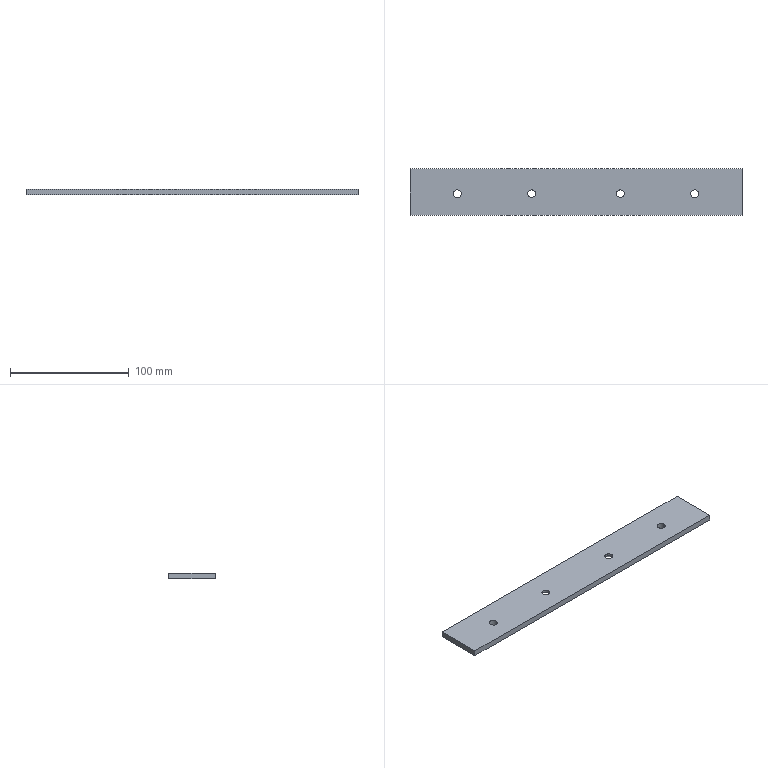Part | STEP file | 44-02-07 Ear Forming Push Plate B | 1 solid | 18 faces | box 280 x 39 x 5 mm | volume 53633 mm3 | cylinder 8 | plane 6 | cone 4 | commonest cylinder face diameters 6.6 x4 6.8 x4
STEP:
#1=CARTESIAN_POINT('',(0.,0.,0.));
#2=DIRECTION('',(0.,0.,1.));
#3=DIRECTION('',(1.,0.,0.));
#4=AXIS2_PLACEMENT_3D('',#1,#2,#3);
#5=CARTESIAN_POINT('',(34.2,0.,0.6));
#6=VERTEX_POINT('',#5);
#7=CARTESIAN_POINT('',(31.1,0.,-2.5));
#8=VERTEX_POINT('',#7);
#9=CARTESIAN_POINT('',(31.1,0.,-2.5));
#10=DIRECTION('',(-0.7071,0.,-0.7071));
#11=VECTOR('',#10,1.);
#12=LINE('',#9,#11);
#13=CARTESIAN_POINT('',(37.5,0.,-2.5));
#14=DIRECTION('',(0.,0.,-1.));
#15=DIRECTION('',(-1.,0.,0.));
#16=AXIS2_PLACEMENT_3D('',#13,#14,#15);
#17=CONICAL_SURFACE('',#16,6.4,0.7854);
#18=CARTESIAN_POINT('',(6.283,0.));
#19=DIRECTION('',(0.,1.));
#20=VECTOR('',#19,1.);
#21=LINE('',#18,#20);
#22=(GEOMETRIC_REPRESENTATION_CONTEXT(2)PARAMETRIC_REPRESENTATION_CONTEXT()REPRESENTATION_CONTEXT('',''));
#23=DEFINITIONAL_REPRESENTATION('',(#21),#22);
#24=PCURVE('',#17,#23);
#25=CARTESIAN_POINT('',(37.5,0.,-2.5));
#26=DIRECTION('',(0.,0.,-1.));
#27=DIRECTION('',(-1.,0.,0.));
#28=AXIS2_PLACEMENT_3D('',#25,#26,#27);
#29=CONICAL_SURFACE('',#28,6.4,0.7854);
#30=CARTESIAN_POINT('',(0.,0.));
#31=DIRECTION('',(0.,1.));
#32=VECTOR('',#31,1.);
#33=LINE('',#30,#32);
#34=(GEOMETRIC_REPRESENTATION_CONTEXT(2)PARAMETRIC_REPRESENTATION_CONTEXT()REPRESENTATION_CONTEXT('',''));
#35=DEFINITIONAL_REPRESENTATION('',(#33),#34);
#36=PCURVE('',#29,#35);
#37=SURFACE_CURVE('',#12,(#24,#36),.PCURVE_S1.);
#38=EDGE_CURVE('',#6,#8,#37,.T.);
#39=ORIENTED_EDGE('',*,*,#38,.T.);
#40=CARTESIAN_POINT('',(43.9,0.,-2.5));
#41=VERTEX_POINT('',#40);
#42=CARTESIAN_POINT('',(37.5,0.,-2.5));
#43=DIRECTION('',(0.,0.,-1.));
#44=DIRECTION('',(-1.,0.,0.));
#45=AXIS2_PLACEMENT_3D('',#42,#43,#44);
#46=CIRCLE('',#45,6.4);
#47=CARTESIAN_POINT('',(0.,0.));
#48=DIRECTION('',(1.,0.));
#49=VECTOR('',#48,1.);
#50=LINE('',#47,#49);
#51=(GEOMETRIC_REPRESENTATION_CONTEXT(2)PARAMETRIC_REPRESENTATION_CONTEXT()REPRESENTATION_CONTEXT('',''));
#52=DEFINITIONAL_REPRESENTATION('',(#50),#51);
#53=PCURVE('',#17,#52);
#54=CARTESIAN_POINT('',(140.,-18.,-2.5));
#55=DIRECTION('',(0.,0.,1.));
#56=DIRECTION('',(1.,0.,0.));
#57=AXIS2_PLACEMENT_3D('',#54,#55,#56);
#58=PLANE('',#57);
#59=CARTESIAN_POINT('',(-108.9,18.));
#60=CARTESIAN_POINT('',(-108.9,29.085));
#61=CARTESIAN_POINT('',(-99.3,23.543));
#62=CARTESIAN_POINT('',(-89.7,18.));
#63=CARTESIAN_POINT('',(-99.3,12.457));
#64=CARTESIAN_POINT('',(-108.9,6.915));
#65=CARTESIAN_POINT('',(-108.9,18.));
#66=(BOUNDED_CURVE()B_SPLINE_CURVE(2,(#59,#60,#61,#62,#63,#64,#65),.UNSPECIFIED.,.T.,.F.)B_SPLINE_CURVE_WITH_KNOTS((1,2,2,2,2,1),(-2.094,0.,2.094,4.189,6.283,8.378),.UNSPECIFIED.)CURVE()GEOMETRIC_REPRESENTATION_ITEM()RATIONAL_B_SPLINE_CURVE((1.,0.5,1.,0.5,1.,0.5,1.))REPRESENTATION_ITEM(''));
#67=(GEOMETRIC_REPRESENTATION_CONTEXT(2)PARAMETRIC_REPRESENTATION_CONTEXT()REPRESENTATION_CONTEXT('',''));
#68=DEFINITIONAL_REPRESENTATION('',(#66),#67);
#69=PCURVE('',#58,#68);
#70=SURFACE_CURVE('',#46,(#53,#69),.PCURVE_S1.);
#71=EDGE_CURVE('',#41,#8,#70,.T.);
#72=ORIENTED_EDGE('',*,*,#71,.F.);
#73=CARTESIAN_POINT('',(40.8,0.,0.6));
#74=VERTEX_POINT('',#73);
#75=CARTESIAN_POINT('',(43.9,0.,-2.5));
#76=DIRECTION('',(0.7071,0.,-0.7071));
#77=VECTOR('',#76,1.);
#78=LINE('',#75,#77);
#79=CARTESIAN_POINT('',(3.142,0.));
#80=DIRECTION('',(0.,1.));
#81=VECTOR('',#80,1.);
#82=LINE('',#79,#81);
#83=(GEOMETRIC_REPRESENTATION_CONTEXT(2)PARAMETRIC_REPRESENTATION_CONTEXT()REPRESENTATION_CONTEXT('',''));
#84=DEFINITIONAL_REPRESENTATION('',(#82),#83);
#85=PCURVE('',#17,#84);
#86=CARTESIAN_POINT('',(3.142,0.));
#87=DIRECTION('',(0.,1.));
#88=VECTOR('',#87,1.);
#89=LINE('',#86,#88);
#90=(GEOMETRIC_REPRESENTATION_CONTEXT(2)PARAMETRIC_REPRESENTATION_CONTEXT()REPRESENTATION_CONTEXT('',''));
#91=DEFINITIONAL_REPRESENTATION('',(#89),#90);
#92=PCURVE('',#29,#91);
#93=SURFACE_CURVE('',#78,(#85,#92),.PCURVE_S1.);
#94=EDGE_CURVE('',#74,#41,#93,.T.);
#95=ORIENTED_EDGE('',*,*,#94,.F.);
#96=CARTESIAN_POINT('',(37.5,0.,0.6));
#97=DIRECTION('',(0.,0.,-1.));
#98=DIRECTION('',(-1.,0.,0.));
#99=AXIS2_PLACEMENT_3D('',#96,#97,#98);
#100=CIRCLE('',#99,3.3);
#101=CARTESIAN_POINT('',(0.,-3.1));
#102=DIRECTION('',(1.,0.));
#103=VECTOR('',#102,1.);
#104=LINE('',#101,#103);
#105=(GEOMETRIC_REPRESENTATION_CONTEXT(2)PARAMETRIC_REPRESENTATION_CONTEXT()REPRESENTATION_CONTEXT('',''));
#106=DEFINITIONAL_REPRESENTATION('',(#104),#105);
#107=PCURVE('',#17,#106);
#108=CARTESIAN_POINT('',(37.5,0.,-2.5));
#109=DIRECTION('',(0.,0.,-1.));
#110=DIRECTION('',(-1.,0.,0.));
#111=AXIS2_PLACEMENT_3D('',#108,#109,#110);
#112=CYLINDRICAL_SURFACE('',#111,3.3);
#113=CARTESIAN_POINT('',(0.,-3.1));
#114=DIRECTION('',(1.,0.));
#115=VECTOR('',#114,1.);
#116=LINE('',#113,#115);
#117=(GEOMETRIC_REPRESENTATION_CONTEXT(2)PARAMETRIC_REPRESENTATION_CONTEXT()REPRESENTATION_CONTEXT('',''));
#118=DEFINITIONAL_REPRESENTATION('',(#116),#117);
#119=PCURVE('',#112,#118);
#120=SURFACE_CURVE('',#100,(#107,#119),.PCURVE_S1.);
#121=EDGE_CURVE('',#74,#6,#120,.T.);
#122=ORIENTED_EDGE('',*,*,#121,.T.);
#123=EDGE_LOOP('',(#39,#72,#95,#122));
#124=FACE_BOUND('',#123,.F.);
#125=ADVANCED_FACE('',(#124),#17,.F.);
#126=CARTESIAN_POINT('',(34.2,0.,2.5));
#127=VERTEX_POINT('',#126);
#128=CARTESIAN_POINT('',(34.2,0.,-2.5));
#129=DIRECTION('',(0.,0.,-1.));
#130=VECTOR('',#129,1.);
#131=LINE('',#128,#130);
#132=CARTESIAN_POINT('',(6.283,0.));
#133=DIRECTION('',(0.,1.));
#134=VECTOR('',#133,1.);
#135=LINE('',#132,#134);
#136=(GEOMETRIC_REPRESENTATION_CONTEXT(2)PARAMETRIC_REPRESENTATION_CONTEXT()REPRESENTATION_CONTEXT('',''));
#137=DEFINITIONAL_REPRESENTATION('',(#135),#136);
#138=PCURVE('',#112,#137);
#139=CARTESIAN_POINT('',(37.5,0.,-2.5));
#140=DIRECTION('',(0.,0.,-1.));
#141=DIRECTION('',(-1.,0.,0.));
#142=AXIS2_PLACEMENT_3D('',#139,#140,#141);
#143=CYLINDRICAL_SURFACE('',#142,3.3);
#144=CARTESIAN_POINT('',(0.,0.));
#145=DIRECTION('',(0.,1.));
#146=VECTOR('',#145,1.);
#147=LINE('',#144,#146);
#148=(GEOMETRIC_REPRESENTATION_CONTEXT(2)PARAMETRIC_REPRESENTATION_CONTEXT()REPRESENTATION_CONTEXT('',''));
#149=DEFINITIONAL_REPRESENTATION('',(#147),#148);
#150=PCURVE('',#143,#149);
#151=SURFACE_CURVE('',#131,(#138,#150),.PCURVE_S1.);
#152=EDGE_CURVE('',#127,#6,#151,.T.);
#153=ORIENTED_EDGE('',*,*,#152,.T.);
#154=ORIENTED_EDGE('',*,*,#121,.F.);
#155=CARTESIAN_POINT('',(40.8,0.,2.5));
#156=VERTEX_POINT('',#155);
#157=CARTESIAN_POINT('',(40.8,0.,-2.5));
#158=DIRECTION('',(0.,0.,-1.));
#159=VECTOR('',#158,1.);
#160=LINE('',#157,#159);
#161=CARTESIAN_POINT('',(3.142,0.));
#162=DIRECTION('',(0.,1.));
#163=VECTOR('',#162,1.);
#164=LINE('',#161,#163);
#165=(GEOMETRIC_REPRESENTATION_CONTEXT(2)PARAMETRIC_REPRESENTATION_CONTEXT()REPRESENTATION_CONTEXT('',''));
#166=DEFINITIONAL_REPRESENTATION('',(#164),#165);
#167=PCURVE('',#112,#166);
#168=CARTESIAN_POINT('',(3.142,0.));
#169=DIRECTION('',(0.,1.));
#170=VECTOR('',#169,1.);
#171=LINE('',#168,#170);
#172=(GEOMETRIC_REPRESENTATION_CONTEXT(2)PARAMETRIC_REPRESENTATION_CONTEXT()REPRESENTATION_CONTEXT('',''));
#173=DEFINITIONAL_REPRESENTATION('',(#171),#172);
#174=PCURVE('',#143,#173);
#175=SURFACE_CURVE('',#160,(#167,#174),.PCURVE_S1.);
#176=EDGE_CURVE('',#156,#74,#175,.T.);
#177=ORIENTED_EDGE('',*,*,#176,.F.);
#178=CARTESIAN_POINT('',(37.5,0.,2.5));
#179=DIRECTION('',(0.,0.,-1.));
#180=DIRECTION('',(-1.,0.,0.));
#181=AXIS2_PLACEMENT_3D('',#178,#179,#180);
#182=CIRCLE('',#181,3.3);
#183=CARTESIAN_POINT('',(0.,-5.));
#184=DIRECTION('',(1.,0.));
#185=VECTOR('',#184,1.);
#186=LINE('',#183,#185);
#187=(GEOMETRIC_REPRESENTATION_CONTEXT(2)PARAMETRIC_REPRESENTATION_CONTEXT()REPRESENTATION_CONTEXT('',''));
#188=DEFINITIONAL_REPRESENTATION('',(#186),#187);
#189=PCURVE('',#112,#188);
#190=CARTESIAN_POINT('',(140.,-18.,2.5));
#191=DIRECTION('',(0.,0.,1.));
#192=DIRECTION('',(1.,0.,0.));
#193=AXIS2_PLACEMENT_3D('',#190,#191,#192);
#194=PLANE('',#193);
#195=CARTESIAN_POINT('',(-105.8,18.));
#196=CARTESIAN_POINT('',(-105.8,23.716));
#197=CARTESIAN_POINT('',(-100.85,20.858));
#198=CARTESIAN_POINT('',(-95.9,18.));
#199=CARTESIAN_POINT('',(-100.85,15.142));
#200=CARTESIAN_POINT('',(-105.8,12.284));
#201=CARTESIAN_POINT('',(-105.8,18.));
#202=(BOUNDED_CURVE()B_SPLINE_CURVE(2,(#195,#196,#197,#198,#199,#200,#201),.UNSPECIFIED.,.T.,.F.)B_SPLINE_CURVE_WITH_KNOTS((1,2,2,2,2,1),(-2.094,0.,2.094,4.189,6.283,8.378),.UNSPECIFIED.)CURVE()GEOMETRIC_REPRESENTATION_ITEM()RATIONAL_B_SPLINE_CURVE((1.,0.5,1.,0.5,1.,0.5,1.))REPRESENTATION_ITEM(''));
#203=(GEOMETRIC_REPRESENTATION_CONTEXT(2)PARAMETRIC_REPRESENTATION_CONTEXT()REPRESENTATION_CONTEXT('',''));
#204=DEFINITIONAL_REPRESENTATION('',(#202),#203);
#205=PCURVE('',#194,#204);
#206=SURFACE_CURVE('',#182,(#189,#205),.PCURVE_S1.);
#207=EDGE_CURVE('',#156,#127,#206,.T.);
#208=ORIENTED_EDGE('',*,*,#207,.T.);
#209=EDGE_LOOP('',(#153,#154,#177,#208));
#210=FACE_BOUND('',#209,.F.);
#211=ADVANCED_FACE('',(#210),#112,.F.);
#212=CARTESIAN_POINT('',(-40.8,0.,0.6));
#213=VERTEX_POINT('',#212);
#214=CARTESIAN_POINT('',(-43.9,0.,-2.5));
#215=VERTEX_POINT('',#214);
#216=CARTESIAN_POINT('',(-43.9,0.,-2.5));
#217=DIRECTION('',(-0.7071,0.,-0.7071));
#218=VECTOR('',#217,1.);
#219=LINE('',#216,#218);
#220=CARTESIAN_POINT('',(-37.5,0.,-2.5));
#221=DIRECTION('',(0.,0.,-1.));
#222=DIRECTION('',(-1.,0.,0.));
#223=AXIS2_PLACEMENT_3D('',#220,#221,#222);
#224=CONICAL_SURFACE('',#223,6.4,0.7854);
#225=CARTESIAN_POINT('',(6.283,0.));
#226=DIRECTION('',(0.,1.));
#227=VECTOR('',#226,1.);
#228=LINE('',#225,#227);
#229=(GEOMETRIC_REPRESENTATION_CONTEXT(2)PARAMETRIC_REPRESENTATION_CONTEXT()REPRESENTATION_CONTEXT('',''));
#230=DEFINITIONAL_REPRESENTATION('',(#228),#229);
#231=PCURVE('',#224,#230);
#232=CARTESIAN_POINT('',(-37.5,0.,-2.5));
#233=DIRECTION('',(0.,0.,-1.));
#234=DIRECTION('',(-1.,0.,0.));
#235=AXIS2_PLACEMENT_3D('',#232,#233,#234);
#236=CONICAL_SURFACE('',#235,6.4,0.7854);
#237=CARTESIAN_POINT('',(0.,0.));
#238=DIRECTION('',(0.,1.));
#239=VECTOR('',#238,1.);
#240=LINE('',#237,#239);
#241=(GEOMETRIC_REPRESENTATION_CONTEXT(2)PARAMETRIC_REPRESENTATION_CONTEXT()REPRESENTATION_CONTEXT('',''));
#242=DEFINITIONAL_REPRESENTATION('',(#240),#241);
#243=PCURVE('',#236,#242);
#244=SURFACE_CURVE('',#219,(#231,#243),.PCURVE_S1.);
#245=EDGE_CURVE('',#213,#215,#244,.T.);
#246=ORIENTED_EDGE('',*,*,#245,.T.);
#247=CARTESIAN_POINT('',(-31.1,0.,-2.5));
#248=VERTEX_POINT('',#247);
#249=CARTESIAN_POINT('',(-37.5,0.,-2.5));
#250=DIRECTION('',(0.,0.,-1.));
#251=DIRECTION('',(-1.,0.,0.));
#252=AXIS2_PLACEMENT_3D('',#249,#250,#251);
#253=CIRCLE('',#252,6.4);
#254=CARTESIAN_POINT('',(0.,0.));
#255=DIRECTION('',(1.,0.));
#256=VECTOR('',#255,1.);
#257=LINE('',#254,#256);
#258=(GEOMETRIC_REPRESENTATION_CONTEXT(2)PARAMETRIC_REPRESENTATION_CONTEXT()REPRESENTATION_CONTEXT('',''));
#259=DEFINITIONAL_REPRESENTATION('',(#257),#258);
#260=PCURVE('',#224,#259);
#261=CARTESIAN_POINT('',(-183.9,18.));
#262=CARTESIAN_POINT('',(-183.9,29.085));
#263=CARTESIAN_POINT('',(-174.3,23.543));
#264=CARTESIAN_POINT('',(-164.7,18.));
#265=CARTESIAN_POINT('',(-174.3,12.457));
#266=CARTESIAN_POINT('',(-183.9,6.915));
#267=CARTESIAN_POINT('',(-183.9,18.));
#268=(BOUNDED_CURVE()B_SPLINE_CURVE(2,(#261,#262,#263,#264,#265,#266,#267),.UNSPECIFIED.,.T.,.F.)B_SPLINE_CURVE_WITH_KNOTS((1,2,2,2,2,1),(-2.094,0.,2.094,4.189,6.283,8.378),.UNSPECIFIED.)CURVE()GEOMETRIC_REPRESENTATION_ITEM()RATIONAL_B_SPLINE_CURVE((1.,0.5,1.,0.5,1.,0.5,1.))REPRESENTATION_ITEM(''));
#269=(GEOMETRIC_REPRESENTATION_CONTEXT(2)PARAMETRIC_REPRESENTATION_CONTEXT()REPRESENTATION_CONTEXT('',''));
#270=DEFINITIONAL_REPRESENTATION('',(#268),#269);
#271=PCURVE('',#58,#270);
#272=SURFACE_CURVE('',#253,(#260,#271),.PCURVE_S1.);
#273=EDGE_CURVE('',#248,#215,#272,.T.);
#274=ORIENTED_EDGE('',*,*,#273,.F.);
#275=CARTESIAN_POINT('',(-34.2,0.,0.6));
#276=VERTEX_POINT('',#275);
#277=CARTESIAN_POINT('',(-31.1,0.,-2.5));
#278=DIRECTION('',(0.7071,0.,-0.7071));
#279=VECTOR('',#278,1.);
#280=LINE('',#277,#279);
#281=CARTESIAN_POINT('',(3.142,0.));
#282=DIRECTION('',(0.,1.));
#283=VECTOR('',#282,1.);
#284=LINE('',#281,#283);
#285=(GEOMETRIC_REPRESENTATION_CONTEXT(2)PARAMETRIC_REPRESENTATION_CONTEXT()REPRESENTATION_CONTEXT('',''));
#286=DEFINITIONAL_REPRESENTATION('',(#284),#285);
#287=PCURVE('',#224,#286);
#288=CARTESIAN_POINT('',(3.142,0.));
#289=DIRECTION('',(0.,1.));
#290=VECTOR('',#289,1.);
#291=LINE('',#288,#290);
#292=(GEOMETRIC_REPRESENTATION_CONTEXT(2)PARAMETRIC_REPRESENTATION_CONTEXT()REPRESENTATION_CONTEXT('',''));
#293=DEFINITIONAL_REPRESENTATION('',(#291),#292);
#294=PCURVE('',#236,#293);
#295=SURFACE_CURVE('',#280,(#287,#294),.PCURVE_S1.);
#296=EDGE_CURVE('',#276,#248,#295,.T.);
#297=ORIENTED_EDGE('',*,*,#296,.F.);
#298=CARTESIAN_POINT('',(-37.5,0.,0.6));
#299=DIRECTION('',(0.,0.,-1.));
#300=DIRECTION('',(-1.,0.,0.));
#301=AXIS2_PLACEMENT_3D('',#298,#299,#300);
#302=CIRCLE('',#301,3.3);
#303=CARTESIAN_POINT('',(0.,-3.1));
#304=DIRECTION('',(1.,0.));
#305=VECTOR('',#304,1.);
#306=LINE('',#303,#305);
#307=(GEOMETRIC_REPRESENTATION_CONTEXT(2)PARAMETRIC_REPRESENTATION_CONTEXT()REPRESENTATION_CONTEXT('',''));
#308=DEFINITIONAL_REPRESENTATION('',(#306),#307);
#309=PCURVE('',#224,#308);
#310=CARTESIAN_POINT('',(-37.5,0.,-2.5));
#311=DIRECTION('',(0.,0.,-1.));
#312=DIRECTION('',(-1.,0.,0.));
#313=AXIS2_PLACEMENT_3D('',#310,#311,#312);
#314=CYLINDRICAL_SURFACE('',#313,3.3);
#315=CARTESIAN_POINT('',(0.,-3.1));
#316=DIRECTION('',(1.,0.));
#317=VECTOR('',#316,1.);
#318=LINE('',#315,#317);
#319=(GEOMETRIC_REPRESENTATION_CONTEXT(2)PARAMETRIC_REPRESENTATION_CONTEXT()REPRESENTATION_CONTEXT('',''));
#320=DEFINITIONAL_REPRESENTATION('',(#318),#319);
#321=PCURVE('',#314,#320);
#322=SURFACE_CURVE('',#302,(#309,#321),.PCURVE_S1.);
#323=EDGE_CURVE('',#276,#213,#322,.T.);
#324=ORIENTED_EDGE('',*,*,#323,.T.);
#325=EDGE_LOOP('',(#246,#274,#297,#324));
#326=FACE_BOUND('',#325,.F.);
#327=ADVANCED_FACE('',(#326),#224,.F.);
#328=CARTESIAN_POINT('',(-40.8,0.,2.5));
#329=VERTEX_POINT('',#328);
#330=CARTESIAN_POINT('',(-40.8,0.,-2.5));
#331=DIRECTION('',(0.,0.,-1.));
#332=VECTOR('',#331,1.);
#333=LINE('',#330,#332);
#334=CARTESIAN_POINT('',(6.283,0.));
#335=DIRECTION('',(0.,1.));
#336=VECTOR('',#335,1.);
#337=LINE('',#334,#336);
#338=(GEOMETRIC_REPRESENTATION_CONTEXT(2)PARAMETRIC_REPRESENTATION_CONTEXT()REPRESENTATION_CONTEXT('',''));
#339=DEFINITIONAL_REPRESENTATION('',(#337),#338);
#340=PCURVE('',#314,#339);
#341=CARTESIAN_POINT('',(-37.5,0.,-2.5));
#342=DIRECTION('',(0.,0.,-1.));
#343=DIRECTION('',(-1.,0.,0.));
#344=AXIS2_PLACEMENT_3D('',#341,#342,#343);
#345=CYLINDRICAL_SURFACE('',#344,3.3);
#346=CARTESIAN_POINT('',(0.,0.));
#347=DIRECTION('',(0.,1.));
#348=VECTOR('',#347,1.);
#349=LINE('',#346,#348);
#350=(GEOMETRIC_REPRESENTATION_CONTEXT(2)PARAMETRIC_REPRESENTATION_CONTEXT()REPRESENTATION_CONTEXT('',''));
#351=DEFINITIONAL_REPRESENTATION('',(#349),#350);
#352=PCURVE('',#345,#351);
#353=SURFACE_CURVE('',#333,(#340,#352),.PCURVE_S1.);
#354=EDGE_CURVE('',#329,#213,#353,.T.);
#355=ORIENTED_EDGE('',*,*,#354,.T.);
#356=ORIENTED_EDGE('',*,*,#323,.F.);
#357=CARTESIAN_POINT('',(-34.2,0.,2.5));
#358=VERTEX_POINT('',#357);
#359=CARTESIAN_POINT('',(-34.2,0.,-2.5));
#360=DIRECTION('',(0.,0.,-1.));
#361=VECTOR('',#360,1.);
#362=LINE('',#359,#361);
#363=CARTESIAN_POINT('',(3.142,0.));
#364=DIRECTION('',(0.,1.));
#365=VECTOR('',#364,1.);
#366=LINE('',#363,#365);
#367=(GEOMETRIC_REPRESENTATION_CONTEXT(2)PARAMETRIC_REPRESENTATION_CONTEXT()REPRESENTATION_CONTEXT('',''));
#368=DEFINITIONAL_REPRESENTATION('',(#366),#367);
#369=PCURVE('',#314,#368);
#370=CARTESIAN_POINT('',(3.142,0.));
#371=DIRECTION('',(0.,1.));
#372=VECTOR('',#371,1.);
#373=LINE('',#370,#372);
#374=(GEOMETRIC_REPRESENTATION_CONTEXT(2)PARAMETRIC_REPRESENTATION_CONTEXT()REPRESENTATION_CONTEXT('',''));
#375=DEFINITIONAL_REPRESENTATION('',(#373),#374);
#376=PCURVE('',#345,#375);
#377=SURFACE_CURVE('',#362,(#369,#376),.PCURVE_S1.);
#378=EDGE_CURVE('',#358,#276,#377,.T.);
#379=ORIENTED_EDGE('',*,*,#378,.F.);
#380=CARTESIAN_POINT('',(-37.5,0.,2.5));
#381=DIRECTION('',(0.,0.,-1.));
#382=DIRECTION('',(-1.,0.,0.));
#383=AXIS2_PLACEMENT_3D('',#380,#381,#382);
#384=CIRCLE('',#383,3.3);
#385=CARTESIAN_POINT('',(0.,-5.));
#386=DIRECTION('',(1.,0.));
#387=VECTOR('',#386,1.);
#388=LINE('',#385,#387);
#389=(GEOMETRIC_REPRESENTATION_CONTEXT(2)PARAMETRIC_REPRESENTATION_CONTEXT()REPRESENTATION_CONTEXT('',''));
#390=DEFINITIONAL_REPRESENTATION('',(#388),#389);
#391=PCURVE('',#314,#390);
#392=CARTESIAN_POINT('',(-180.8,18.));
#393=CARTESIAN_POINT('',(-180.8,23.716));
#394=CARTESIAN_POINT('',(-175.85,20.858));
#395=CARTESIAN_POINT('',(-170.9,18.));
#396=CARTESIAN_POINT('',(-175.85,15.142));
#397=CARTESIAN_POINT('',(-180.8,12.284));
#398=CARTESIAN_POINT('',(-180.8,18.));
#399=(BOUNDED_CURVE()B_SPLINE_CURVE(2,(#392,#393,#394,#395,#396,#397,#398),.UNSPECIFIED.,.T.,.F.)B_SPLINE_CURVE_WITH_KNOTS((1,2,2,2,2,1),(-2.094,0.,2.094,4.189,6.283,8.378),.UNSPECIFIED.)CURVE()GEOMETRIC_REPRESENTATION_ITEM()RATIONAL_B_SPLINE_CURVE((1.,0.5,1.,0.5,1.,0.5,1.))REPRESENTATION_ITEM(''));
#400=(GEOMETRIC_REPRESENTATION_CONTEXT(2)PARAMETRIC_REPRESENTATION_CONTEXT()REPRESENTATION_CONTEXT('',''));
#401=DEFINITIONAL_REPRESENTATION('',(#399),#400);
#402=PCURVE('',#194,#401);
#403=SURFACE_CURVE('',#384,(#391,#402),.PCURVE_S1.);
#404=EDGE_CURVE('',#358,#329,#403,.T.);
#405=ORIENTED_EDGE('',*,*,#404,.T.);
#406=EDGE_LOOP('',(#355,#356,#379,#405));
#407=FACE_BOUND('',#406,.F.);
#408=ADVANCED_FACE('',(#407),#314,.F.);
#409=CARTESIAN_POINT('',(-103.4,0.,2.5));
#410=VERTEX_POINT('',#409);
#411=CARTESIAN_POINT('',(-103.4,0.,-2.5));
#412=VERTEX_POINT('',#411);
#413=CARTESIAN_POINT('',(-103.4,0.,-2.5));
#414=DIRECTION('',(0.,0.,-1.));
#415=VECTOR('',#414,1.);
#416=LINE('',#413,#415);
#417=CARTESIAN_POINT('',(-100.,0.,-2.5));
#418=DIRECTION('',(0.,0.,-1.));
#419=DIRECTION('',(-1.,0.,0.));
#420=AXIS2_PLACEMENT_3D('',#417,#418,#419);
#421=CYLINDRICAL_SURFACE('',#420,3.4);
#422=CARTESIAN_POINT('',(6.283,0.));
#423=DIRECTION('',(0.,1.));
#424=VECTOR('',#423,1.);
#425=LINE('',#422,#424);
#426=(GEOMETRIC_REPRESENTATION_CONTEXT(2)PARAMETRIC_REPRESENTATION_CONTEXT()REPRESENTATION_CONTEXT('',''));
#427=DEFINITIONAL_REPRESENTATION('',(#425),#426);
#428=PCURVE('',#421,#427);
#429=CARTESIAN_POINT('',(-100.,0.,-2.5));
#430=DIRECTION('',(0.,0.,-1.));
#431=DIRECTION('',(-1.,0.,0.));
#432=AXIS2_PLACEMENT_3D('',#429,#430,#431);
#433=CYLINDRICAL_SURFACE('',#432,3.4);
#434=CARTESIAN_POINT('',(0.,0.));
#435=DIRECTION('',(0.,1.));
#436=VECTOR('',#435,1.);
#437=LINE('',#434,#436);
#438=(GEOMETRIC_REPRESENTATION_CONTEXT(2)PARAMETRIC_REPRESENTATION_CONTEXT()REPRESENTATION_CONTEXT('',''));
#439=DEFINITIONAL_REPRESENTATION('',(#437),#438);
#440=PCURVE('',#433,#439);
#441=SURFACE_CURVE('',#416,(#428,#440),.PCURVE_S1.);
#442=EDGE_CURVE('',#410,#412,#441,.T.);
#443=ORIENTED_EDGE('',*,*,#442,.T.);
#444=CARTESIAN_POINT('',(-96.6,0.,-2.5));
#445=VERTEX_POINT('',#444);
#446=CARTESIAN_POINT('',(-100.,0.,-2.5));
#447=DIRECTION('',(0.,0.,-1.));
#448=DIRECTION('',(-1.,0.,0.));
#449=AXIS2_PLACEMENT_3D('',#446,#447,#448);
#450=CIRCLE('',#449,3.4);
#451=CARTESIAN_POINT('',(0.,0.));
#452=DIRECTION('',(1.,0.));
#453=VECTOR('',#452,1.);
#454=LINE('',#451,#453);
#455=(GEOMETRIC_REPRESENTATION_CONTEXT(2)PARAMETRIC_REPRESENTATION_CONTEXT()REPRESENTATION_CONTEXT('',''));
#456=DEFINITIONAL_REPRESENTATION('',(#454),#455);
#457=PCURVE('',#421,#456);
#458=CARTESIAN_POINT('',(-243.4,18.));
#459=CARTESIAN_POINT('',(-243.4,23.889));
#460=CARTESIAN_POINT('',(-238.3,20.944));
#461=CARTESIAN_POINT('',(-233.2,18.));
#462=CARTESIAN_POINT('',(-238.3,15.056));
#463=CARTESIAN_POINT('',(-243.4,12.111));
#464=CARTESIAN_POINT('',(-243.4,18.));
#465=(BOUNDED_CURVE()B_SPLINE_CURVE(2,(#458,#459,#460,#461,#462,#463,#464),.UNSPECIFIED.,.T.,.F.)B_SPLINE_CURVE_WITH_KNOTS((1,2,2,2,2,1),(-2.094,0.,2.094,4.189,6.283,8.378),.UNSPECIFIED.)CURVE()GEOMETRIC_REPRESENTATION_ITEM()RATIONAL_B_SPLINE_CURVE((1.,0.5,1.,0.5,1.,0.5,1.))REPRESENTATION_ITEM(''));
#466=(GEOMETRIC_REPRESENTATION_CONTEXT(2)PARAMETRIC_REPRESENTATION_CONTEXT()REPRESENTATION_CONTEXT('',''));
#467=DEFINITIONAL_REPRESENTATION('',(#465),#466);
#468=PCURVE('',#58,#467);
#469=SURFACE_CURVE('',#450,(#457,#468),.PCURVE_S1.);
#470=EDGE_CURVE('',#445,#412,#469,.T.);
#471=ORIENTED_EDGE('',*,*,#470,.F.);
#472=CARTESIAN_POINT('',(-96.6,0.,2.5));
#473=VERTEX_POINT('',#472);
#474=CARTESIAN_POINT('',(-96.6,0.,-2.5));
#475=DIRECTION('',(0.,0.,-1.));
#476=VECTOR('',#475,1.);
#477=LINE('',#474,#476);
#478=CARTESIAN_POINT('',(3.142,0.));
#479=DIRECTION('',(0.,1.));
#480=VECTOR('',#479,1.);
#481=LINE('',#478,#480);
#482=(GEOMETRIC_REPRESENTATION_CONTEXT(2)PARAMETRIC_REPRESENTATION_CONTEXT()REPRESENTATION_CONTEXT('',''));
#483=DEFINITIONAL_REPRESENTATION('',(#481),#482);
#484=PCURVE('',#421,#483);
#485=CARTESIAN_POINT('',(3.142,0.));
#486=DIRECTION('',(0.,1.));
#487=VECTOR('',#486,1.);
#488=LINE('',#485,#487);
#489=(GEOMETRIC_REPRESENTATION_CONTEXT(2)PARAMETRIC_REPRESENTATION_CONTEXT()REPRESENTATION_CONTEXT('',''));
#490=DEFINITIONAL_REPRESENTATION('',(#488),#489);
#491=PCURVE('',#433,#490);
#492=SURFACE_CURVE('',#477,(#484,#491),.PCURVE_S1.);
#493=EDGE_CURVE('',#473,#445,#492,.T.);
#494=ORIENTED_EDGE('',*,*,#493,.F.);
#495=CARTESIAN_POINT('',(-100.,0.,2.5));
#496=DIRECTION('',(0.,0.,-1.));
#497=DIRECTION('',(-1.,0.,0.));
#498=AXIS2_PLACEMENT_3D('',#495,#496,#497);
#499=CIRCLE('',#498,3.4);
#500=CARTESIAN_POINT('',(0.,-5.));
#501=DIRECTION('',(1.,0.));
#502=VECTOR('',#501,1.);
#503=LINE('',#500,#502);
#504=(GEOMETRIC_REPRESENTATION_CONTEXT(2)PARAMETRIC_REPRESENTATION_CONTEXT()REPRESENTATION_CONTEXT('',''));
#505=DEFINITIONAL_REPRESENTATION('',(#503),#504);
#506=PCURVE('',#421,#505);
#507=CARTESIAN_POINT('',(-243.4,18.));
#508=CARTESIAN_POINT('',(-243.4,23.889));
#509=CARTESIAN_POINT('',(-238.3,20.944));
#510=CARTESIAN_POINT('',(-233.2,18.));
#511=CARTESIAN_POINT('',(-238.3,15.056));
#512=CARTESIAN_POINT('',(-243.4,12.111));
#513=CARTESIAN_POINT('',(-243.4,18.));
#514=(BOUNDED_CURVE()B_SPLINE_CURVE(2,(#507,#508,#509,#510,#511,#512,#513),.UNSPECIFIED.,.T.,.F.)B_SPLINE_CURVE_WITH_KNOTS((1,2,2,2,2,1),(-2.094,0.,2.094,4.189,6.283,8.378),.UNSPECIFIED.)CURVE()GEOMETRIC_REPRESENTATION_ITEM()RATIONAL_B_SPLINE_CURVE((1.,0.5,1.,0.5,1.,0.5,1.))REPRESENTATION_ITEM(''));
#515=(GEOMETRIC_REPRESENTATION_CONTEXT(2)PARAMETRIC_REPRESENTATION_CONTEXT()REPRESENTATION_CONTEXT('',''));
#516=DEFINITIONAL_REPRESENTATION('',(#514),#515);
#517=PCURVE('',#194,#516);
#518=SURFACE_CURVE('',#499,(#506,#517),.PCURVE_S1.);
#519=EDGE_CURVE('',#473,#410,#518,.T.);
#520=ORIENTED_EDGE('',*,*,#519,.T.);
#521=EDGE_LOOP('',(#443,#471,#494,#520));
#522=FACE_BOUND('',#521,.F.);
#523=ADVANCED_FACE('',(#522),#421,.F.);
#524=CARTESIAN_POINT('',(96.6,0.,2.5));
#525=VERTEX_POINT('',#524);
#526=CARTESIAN_POINT('',(96.6,0.,-2.5));
#527=VERTEX_POINT('',#526);
#528=CARTESIAN_POINT('',(96.6,0.,-2.5));
#529=DIRECTION('',(0.,0.,-1.));
#530=VECTOR('',#529,1.);
#531=LINE('',#528,#530);
#532=CARTESIAN_POINT('',(100.,0.,-2.5));
#533=DIRECTION('',(0.,0.,-1.));
#534=DIRECTION('',(-1.,0.,0.));
#535=AXIS2_PLACEMENT_3D('',#532,#533,#534);
#536=CYLINDRICAL_SURFACE('',#535,3.4);
#537=CARTESIAN_POINT('',(6.283,0.));
#538=DIRECTION('',(0.,1.));
#539=VECTOR('',#538,1.);
#540=LINE('',#537,#539);
#541=(GEOMETRIC_REPRESENTATION_CONTEXT(2)PARAMETRIC_REPRESENTATION_CONTEXT()REPRESENTATION_CONTEXT('',''));
#542=DEFINITIONAL_REPRESENTATION('',(#540),#541);
#543=PCURVE('',#536,#542);
#544=CARTESIAN_POINT('',(100.,0.,-2.5));
#545=DIRECTION('',(0.,0.,-1.));
#546=DIRECTION('',(-1.,0.,0.));
#547=AXIS2_PLACEMENT_3D('',#544,#545,#546);
#548=CYLINDRICAL_SURFACE('',#547,3.4);
#549=CARTESIAN_POINT('',(0.,0.));
#550=DIRECTION('',(0.,1.));
#551=VECTOR('',#550,1.);
#552=LINE('',#549,#551);
#553=(GEOMETRIC_REPRESENTATION_CONTEXT(2)PARAMETRIC_REPRESENTATION_CONTEXT()REPRESENTATION_CONTEXT('',''));
#554=DEFINITIONAL_REPRESENTATION('',(#552),#553);
#555=PCURVE('',#548,#554);
#556=SURFACE_CURVE('',#531,(#543,#555),.PCURVE_S1.);
#557=EDGE_CURVE('',#525,#527,#556,.T.);
#558=ORIENTED_EDGE('',*,*,#557,.T.);
#559=CARTESIAN_POINT('',(103.4,0.,-2.5));
#560=VERTEX_POINT('',#559);
#561=CARTESIAN_POINT('',(100.,0.,-2.5));
#562=DIRECTION('',(0.,0.,-1.));
#563=DIRECTION('',(-1.,0.,0.));
#564=AXIS2_PLACEMENT_3D('',#561,#562,#563);
#565=CIRCLE('',#564,3.4);
#566=CARTESIAN_POINT('',(0.,0.));
#567=DIRECTION('',(1.,0.));
#568=VECTOR('',#567,1.);
#569=LINE('',#566,#568);
#570=(GEOMETRIC_REPRESENTATION_CONTEXT(2)PARAMETRIC_REPRESENTATION_CONTEXT()REPRESENTATION_CONTEXT('',''));
#571=DEFINITIONAL_REPRESENTATION('',(#569),#570);
#572=PCURVE('',#536,#571);
#573=CARTESIAN_POINT('',(-43.4,18.));
#574=CARTESIAN_POINT('',(-43.4,23.889));
#575=CARTESIAN_POINT('',(-38.3,20.944));
#576=CARTESIAN_POINT('',(-33.2,18.));
#577=CARTESIAN_POINT('',(-38.3,15.056));
#578=CARTESIAN_POINT('',(-43.4,12.111));
#579=CARTESIAN_POINT('',(-43.4,18.));
#580=(BOUNDED_CURVE()B_SPLINE_CURVE(2,(#573,#574,#575,#576,#577,#578,#579),.UNSPECIFIED.,.T.,.F.)B_SPLINE_CURVE_WITH_KNOTS((1,2,2,2,2,1),(-2.094,0.,2.094,4.189,6.283,8.378),.UNSPECIFIED.)CURVE()GEOMETRIC_REPRESENTATION_ITEM()RATIONAL_B_SPLINE_CURVE((1.,0.5,1.,0.5,1.,0.5,1.))REPRESENTATION_ITEM(''));
#581=(GEOMETRIC_REPRESENTATION_CONTEXT(2)PARAMETRIC_REPRESENTATION_CONTEXT()REPRESENTATION_CONTEXT('',''));
#582=DEFINITIONAL_REPRESENTATION('',(#580),#581);
#583=PCURVE('',#58,#582);
#584=SURFACE_CURVE('',#565,(#572,#583),.PCURVE_S1.);
#585=EDGE_CURVE('',#560,#527,#584,.T.);
#586=ORIENTED_EDGE('',*,*,#585,.F.);
#587=CARTESIAN_POINT('',(103.4,0.,2.5));
#588=VERTEX_POINT('',#587);
#589=CARTESIAN_POINT('',(103.4,0.,-2.5));
#590=DIRECTION('',(0.,0.,-1.));
#591=VECTOR('',#590,1.);
#592=LINE('',#589,#591);
#593=CARTESIAN_POINT('',(3.142,0.));
#594=DIRECTION('',(0.,1.));
#595=VECTOR('',#594,1.);
#596=LINE('',#593,#595);
#597=(GEOMETRIC_REPRESENTATION_CONTEXT(2)PARAMETRIC_REPRESENTATION_CONTEXT()REPRESENTATION_CONTEXT('',''));
#598=DEFINITIONAL_REPRESENTATION('',(#596),#597);
#599=PCURVE('',#536,#598);
#600=CARTESIAN_POINT('',(3.142,0.));
#601=DIRECTION('',(0.,1.));
#602=VECTOR('',#601,1.);
#603=LINE('',#600,#602);
#604=(GEOMETRIC_REPRESENTATION_CONTEXT(2)PARAMETRIC_REPRESENTATION_CONTEXT()REPRESENTATION_CONTEXT('',''));
#605=DEFINITIONAL_REPRESENTATION('',(#603),#604);
#606=PCURVE('',#548,#605);
#607=SURFACE_CURVE('',#592,(#599,#606),.PCURVE_S1.);
#608=EDGE_CURVE('',#588,#560,#607,.T.);
#609=ORIENTED_EDGE('',*,*,#608,.F.);
#610=CARTESIAN_POINT('',(100.,0.,2.5));
#611=DIRECTION('',(0.,0.,-1.));
#612=DIRECTION('',(-1.,0.,0.));
#613=AXIS2_PLACEMENT_3D('',#610,#611,#612);
#614=CIRCLE('',#613,3.4);
#615=CARTESIAN_POINT('',(0.,-5.));
#616=DIRECTION('',(1.,0.));
#617=VECTOR('',#616,1.);
#618=LINE('',#615,#617);
#619=(GEOMETRIC_REPRESENTATION_CONTEXT(2)PARAMETRIC_REPRESENTATION_CONTEXT()REPRESENTATION_CONTEXT('',''));
#620=DEFINITIONAL_REPRESENTATION('',(#618),#619);
#621=PCURVE('',#536,#620);
#622=CARTESIAN_POINT('',(-43.4,18.));
#623=CARTESIAN_POINT('',(-43.4,23.889));
#624=CARTESIAN_POINT('',(-38.3,20.944));
#625=CARTESIAN_POINT('',(-33.2,18.));
#626=CARTESIAN_POINT('',(-38.3,15.056));
#627=CARTESIAN_POINT('',(-43.4,12.111));
#628=CARTESIAN_POINT('',(-43.4,18.));
#629=(BOUNDED_CURVE()B_SPLINE_CURVE(2,(#622,#623,#624,#625,#626,#627,#628),.UNSPECIFIED.,.T.,.F.)B_SPLINE_CURVE_WITH_KNOTS((1,2,2,2,2,1),(-2.094,0.,2.094,4.189,6.283,8.378),.UNSPECIFIED.)CURVE()GEOMETRIC_REPRESENTATION_ITEM()RATIONAL_B_SPLINE_CURVE((1.,0.5,1.,0.5,1.,0.5,1.))REPRESENTATION_ITEM(''));
#630=(GEOMETRIC_REPRESENTATION_CONTEXT(2)PARAMETRIC_REPRESENTATION_CONTEXT()REPRESENTATION_CONTEXT('',''));
#631=DEFINITIONAL_REPRESENTATION('',(#629),#630);
#632=PCURVE('',#194,#631);
#633=SURFACE_CURVE('',#614,(#621,#632),.PCURVE_S1.);
#634=EDGE_CURVE('',#588,#525,#633,.T.);
#635=ORIENTED_EDGE('',*,*,#634,.T.);
#636=EDGE_LOOP('',(#558,#586,#609,#635));
#637=FACE_BOUND('',#636,.F.);
#638=ADVANCED_FACE('',(#637),#536,.F.);
#639=CARTESIAN_POINT('',(140.,-18.,-2.5));
#640=VERTEX_POINT('',#639);
#641=CARTESIAN_POINT('',(140.,21.,-2.5));
#642=VERTEX_POINT('',#641);
#643=CARTESIAN_POINT('',(140.,18.,-2.5));
#644=DIRECTION('',(0.,1.,0.));
#645=VECTOR('',#644,1.);
#646=LINE('',#643,#645);
#647=CARTESIAN_POINT('',(140.,18.,2.5));
#648=DIRECTION('',(-1.,0.,0.));
#649=DIRECTION('',(0.,0.,1.));
#650=AXIS2_PLACEMENT_3D('',#647,#648,#649);
#651=PLANE('',#650);
#652=CARTESIAN_POINT('',(-5.,0.));
#653=DIRECTION('',(0.,1.));
#654=VECTOR('',#653,1.);
#655=LINE('',#652,#654);
#656=(GEOMETRIC_REPRESENTATION_CONTEXT(2)PARAMETRIC_REPRESENTATION_CONTEXT()REPRESENTATION_CONTEXT('',''));
#657=DEFINITIONAL_REPRESENTATION('',(#655),#656);
#658=PCURVE('',#651,#657);
#659=CARTESIAN_POINT('',(0.,36.));
#660=DIRECTION('',(0.,1.));
#661=VECTOR('',#660,1.);
#662=LINE('',#659,#661);
#663=(GEOMETRIC_REPRESENTATION_CONTEXT(2)PARAMETRIC_REPRESENTATION_CONTEXT()REPRESENTATION_CONTEXT('',''));
#664=DEFINITIONAL_REPRESENTATION('',(#662),#663);
#665=PCURVE('',#58,#664);
#666=SURFACE_CURVE('',#646,(#658,#665),.PCURVE_S1.);
#667=EDGE_CURVE('',#640,#642,#666,.T.);
#668=ORIENTED_EDGE('',*,*,#667,.T.);
#669=CARTESIAN_POINT('',(140.,21.,2.5));
#670=VERTEX_POINT('',#669);
#671=CARTESIAN_POINT('',(140.,21.,-2.5));
#672=DIRECTION('',(0.,0.,-1.));
#673=VECTOR('',#672,1.);
#674=LINE('',#671,#673);
#675=CARTESIAN_POINT('',(-5.,3.));
#676=DIRECTION('',(-1.,0.));
#677=VECTOR('',#676,1.);
#678=LINE('',#675,#677);
#679=(GEOMETRIC_REPRESENTATION_CONTEXT(2)PARAMETRIC_REPRESENTATION_CONTEXT()REPRESENTATION_CONTEXT('',''));
#680=DEFINITIONAL_REPRESENTATION('',(#678),#679);
#681=PCURVE('',#651,#680);
#682=CARTESIAN_POINT('',(-140.,21.,2.5));
#683=DIRECTION('',(0.,1.,0.));
#684=DIRECTION('',(0.,0.,1.));
#685=AXIS2_PLACEMENT_3D('',#682,#683,#684);
#686=PLANE('',#685);
#687=CARTESIAN_POINT('',(-5.,280.));
#688=DIRECTION('',(-1.,0.));
#689=VECTOR('',#688,1.);
#690=LINE('',#687,#689);
#691=(GEOMETRIC_REPRESENTATION_CONTEXT(2)PARAMETRIC_REPRESENTATION_CONTEXT()REPRESENTATION_CONTEXT('',''));
#692=DEFINITIONAL_REPRESENTATION('',(#690),#691);
#693=PCURVE('',#686,#692);
#694=SURFACE_CURVE('',#674,(#681,#693),.PCURVE_S1.);
#695=EDGE_CURVE('',#670,#642,#694,.T.);
#696=ORIENTED_EDGE('',*,*,#695,.F.);
#697=CARTESIAN_POINT('',(140.,-18.,2.5));
#698=VERTEX_POINT('',#697);
#699=CARTESIAN_POINT('',(140.,18.,2.5));
#700=DIRECTION('',(0.,1.,0.));
#701=VECTOR('',#700,1.);
#702=LINE('',#699,#701);
#703=CARTESIAN_POINT('',(0.,0.));
#704=DIRECTION('',(0.,1.));
#705=VECTOR('',#704,1.);
#706=LINE('',#703,#705);
#707=(GEOMETRIC_REPRESENTATION_CONTEXT(2)PARAMETRIC_REPRESENTATION_CONTEXT()REPRESENTATION_CONTEXT('',''));
#708=DEFINITIONAL_REPRESENTATION('',(#706),#707);
#709=PCURVE('',#651,#708);
#710=CARTESIAN_POINT('',(0.,36.));
#711=DIRECTION('',(0.,1.));
#712=VECTOR('',#711,1.);
#713=LINE('',#710,#712);
#714=(GEOMETRIC_REPRESENTATION_CONTEXT(2)PARAMETRIC_REPRESENTATION_CONTEXT()REPRESENTATION_CONTEXT('',''));
#715=DEFINITIONAL_REPRESENTATION('',(#713),#714);
#716=PCURVE('',#194,#715);
#717=SURFACE_CURVE('',#702,(#709,#716),.PCURVE_S1.);
#718=EDGE_CURVE('',#698,#670,#717,.T.);
#719=ORIENTED_EDGE('',*,*,#718,.F.);
#720=CARTESIAN_POINT('',(140.,-18.,2.5));
#721=DIRECTION('',(0.,0.,-1.));
#722=VECTOR('',#721,1.);
#723=LINE('',#720,#722);
#724=CARTESIAN_POINT('',(0.,-36.));
#725=DIRECTION('',(-1.,0.));
#726=VECTOR('',#725,1.);
#727=LINE('',#724,#726);
#728=(GEOMETRIC_REPRESENTATION_CONTEXT(2)PARAMETRIC_REPRESENTATION_CONTEXT()REPRESENTATION_CONTEXT('',''));
#729=DEFINITIONAL_REPRESENTATION('',(#727),#728);
#730=PCURVE('',#651,#729);
#731=CARTESIAN_POINT('',(-140.,-18.,2.5));
#732=DIRECTION('',(0.,1.,0.));
#733=DIRECTION('',(0.,0.,1.));
#734=AXIS2_PLACEMENT_3D('',#731,#732,#733);
#735=PLANE('',#734);
#736=CARTESIAN_POINT('',(0.,280.));
#737=DIRECTION('',(-1.,0.));
#738=VECTOR('',#737,1.);
#739=LINE('',#736,#738);
#740=(GEOMETRIC_REPRESENTATION_CONTEXT(2)PARAMETRIC_REPRESENTATION_CONTEXT()REPRESENTATION_CONTEXT('',''));
#741=DEFINITIONAL_REPRESENTATION('',(#739),#740);
#742=PCURVE('',#735,#741);
#743=SURFACE_CURVE('',#723,(#730,#742),.PCURVE_S1.);
#744=EDGE_CURVE('',#698,#640,#743,.T.);
#745=ORIENTED_EDGE('',*,*,#744,.T.);
#746=EDGE_LOOP('',(#668,#696,#719,#745));
#747=FACE_BOUND('',#746,.T.);
#748=ADVANCED_FACE('',(#747),#651,.F.);
#749=CARTESIAN_POINT('',(-140.,21.,-2.5));
#750=VERTEX_POINT('',#749);
#751=CARTESIAN_POINT('',(-140.,-18.,-2.5));
#752=VERTEX_POINT('',#751);
#753=CARTESIAN_POINT('',(-140.,18.,-2.5));
#754=DIRECTION('',(0.,-1.,0.));
#755=VECTOR('',#754,1.);
#756=LINE('',#753,#755);
#757=CARTESIAN_POINT('',(-140.,18.,2.5));
#758=DIRECTION('',(1.,0.,0.));
#759=DIRECTION('',(0.,0.,-1.));
#760=AXIS2_PLACEMENT_3D('',#757,#758,#759);
#761=PLANE('',#760);
#762=CARTESIAN_POINT('',(5.,0.));
#763=DIRECTION('',(0.,-1.));
#764=VECTOR('',#763,1.);
#765=LINE('',#762,#764);
#766=(GEOMETRIC_REPRESENTATION_CONTEXT(2)PARAMETRIC_REPRESENTATION_CONTEXT()REPRESENTATION_CONTEXT('',''));
#767=DEFINITIONAL_REPRESENTATION('',(#765),#766);
#768=PCURVE('',#761,#767);
#769=CARTESIAN_POINT('',(-280.,36.));
#770=DIRECTION('',(0.,-1.));
#771=VECTOR('',#770,1.);
#772=LINE('',#769,#771);
#773=(GEOMETRIC_REPRESENTATION_CONTEXT(2)PARAMETRIC_REPRESENTATION_CONTEXT()REPRESENTATION_CONTEXT('',''));
#774=DEFINITIONAL_REPRESENTATION('',(#772),#773);
#775=PCURVE('',#58,#774);
#776=SURFACE_CURVE('',#756,(#768,#775),.PCURVE_S1.);
#777=EDGE_CURVE('',#750,#752,#776,.T.);
#778=ORIENTED_EDGE('',*,*,#777,.T.);
#779=CARTESIAN_POINT('',(-140.,-18.,2.5));
#780=VERTEX_POINT('',#779);
#781=CARTESIAN_POINT('',(-140.,-18.,2.5));
#782=DIRECTION('',(0.,0.,-1.));
#783=VECTOR('',#782,1.);
#784=LINE('',#781,#783);
#785=CARTESIAN_POINT('',(0.,-36.));
#786=DIRECTION('',(1.,0.));
#787=VECTOR('',#786,1.);
#788=LINE('',#785,#787);
#789=(GEOMETRIC_REPRESENTATION_CONTEXT(2)PARAMETRIC_REPRESENTATION_CONTEXT()REPRESENTATION_CONTEXT('',''));
#790=DEFINITIONAL_REPRESENTATION('',(#788),#789);
#791=PCURVE('',#761,#790);
#792=CARTESIAN_POINT('',(0.,0.));
#793=DIRECTION('',(-1.,0.));
#794=VECTOR('',#793,1.);
#795=LINE('',#792,#794);
#796=(GEOMETRIC_REPRESENTATION_CONTEXT(2)PARAMETRIC_REPRESENTATION_CONTEXT()REPRESENTATION_CONTEXT('',''));
#797=DEFINITIONAL_REPRESENTATION('',(#795),#796);
#798=PCURVE('',#735,#797);
#799=SURFACE_CURVE('',#784,(#791,#798),.PCURVE_S1.);
#800=EDGE_CURVE('',#780,#752,#799,.T.);
#801=ORIENTED_EDGE('',*,*,#800,.F.);
#802=CARTESIAN_POINT('',(-140.,21.,2.5));
#803=VERTEX_POINT('',#802);
#804=CARTESIAN_POINT('',(-140.,18.,2.5));
#805=DIRECTION('',(0.,-1.,0.));
#806=VECTOR('',#805,1.);
#807=LINE('',#804,#806);
#808=CARTESIAN_POINT('',(0.,0.));
#809=DIRECTION('',(0.,-1.));
#810=VECTOR('',#809,1.);
#811=LINE('',#808,#810);
#812=(GEOMETRIC_REPRESENTATION_CONTEXT(2)PARAMETRIC_REPRESENTATION_CONTEXT()REPRESENTATION_CONTEXT('',''));
#813=DEFINITIONAL_REPRESENTATION('',(#811),#812);
#814=PCURVE('',#761,#813);
#815=CARTESIAN_POINT('',(-280.,36.));
#816=DIRECTION('',(0.,-1.));
#817=VECTOR('',#816,1.);
#818=LINE('',#815,#817);
#819=(GEOMETRIC_REPRESENTATION_CONTEXT(2)PARAMETRIC_REPRESENTATION_CONTEXT()REPRESENTATION_CONTEXT('',''));
#820=DEFINITIONAL_REPRESENTATION('',(#818),#819);
#821=PCURVE('',#194,#820);
#822=SURFACE_CURVE('',#807,(#814,#821),.PCURVE_S1.);
#823=EDGE_CURVE('',#803,#780,#822,.T.);
#824=ORIENTED_EDGE('',*,*,#823,.F.);
#825=CARTESIAN_POINT('',(-140.,21.,-2.5));
#826=DIRECTION('',(0.,0.,1.));
#827=VECTOR('',#826,1.);
#828=LINE('',#825,#827);
#829=CARTESIAN_POINT('',(5.,3.));
#830=DIRECTION('',(-1.,0.));
#831=VECTOR('',#830,1.);
#832=LINE('',#829,#831);
#833=(GEOMETRIC_REPRESENTATION_CONTEXT(2)PARAMETRIC_REPRESENTATION_CONTEXT()REPRESENTATION_CONTEXT('',''));
#834=DEFINITIONAL_REPRESENTATION('',(#832),#833);
#835=PCURVE('',#761,#834);
#836=CARTESIAN_POINT('',(-5.,0.));
#837=DIRECTION('',(1.,0.));
#838=VECTOR('',#837,1.);
#839=LINE('',#836,#838);
#840=(GEOMETRIC_REPRESENTATION_CONTEXT(2)PARAMETRIC_REPRESENTATION_CONTEXT()REPRESENTATION_CONTEXT('',''));
#841=DEFINITIONAL_REPRESENTATION('',(#839),#840);
#842=PCURVE('',#686,#841);
#843=SURFACE_CURVE('',#828,(#835,#842),.PCURVE_S1.);
#844=EDGE_CURVE('',#750,#803,#843,.T.);
#845=ORIENTED_EDGE('',*,*,#844,.F.);
#846=EDGE_LOOP('',(#778,#801,#824,#845));
#847=FACE_BOUND('',#846,.T.);
#848=ADVANCED_FACE('',(#847),#761,.F.);
#849=CARTESIAN_POINT('',(-140.,-18.,-2.5));
#850=DIRECTION('',(1.,0.,0.));
#851=VECTOR('',#850,1.);
#852=LINE('',#849,#851);
#853=CARTESIAN_POINT('',(-5.,0.));
#854=DIRECTION('',(0.,1.));
#855=VECTOR('',#854,1.);
#856=LINE('',#853,#855);
#857=(GEOMETRIC_REPRESENTATION_CONTEXT(2)PARAMETRIC_REPRESENTATION_CONTEXT()REPRESENTATION_CONTEXT('',''));
#858=DEFINITIONAL_REPRESENTATION('',(#856),#857);
#859=PCURVE('',#735,#858);
#860=CARTESIAN_POINT('',(-280.,0.));
#861=DIRECTION('',(1.,0.));
#862=VECTOR('',#861,1.);
#863=LINE('',#860,#862);
#864=(GEOMETRIC_REPRESENTATION_CONTEXT(2)PARAMETRIC_REPRESENTATION_CONTEXT()REPRESENTATION_CONTEXT('',''));
#865=DEFINITIONAL_REPRESENTATION('',(#863),#864);
#866=PCURVE('',#58,#865);
#867=SURFACE_CURVE('',#852,(#859,#866),.PCURVE_S1.);
#868=EDGE_CURVE('',#752,#640,#867,.T.);
#869=ORIENTED_EDGE('',*,*,#868,.T.);
#870=ORIENTED_EDGE('',*,*,#744,.F.);
#871=CARTESIAN_POINT('',(-140.,-18.,2.5));
#872=DIRECTION('',(1.,0.,0.));
#873=VECTOR('',#872,1.);
#874=LINE('',#871,#873);
#875=CARTESIAN_POINT('',(0.,0.));
#876=DIRECTION('',(0.,1.));
#877=VECTOR('',#876,1.);
#878=LINE('',#875,#877);
#879=(GEOMETRIC_REPRESENTATION_CONTEXT(2)PARAMETRIC_REPRESENTATION_CONTEXT()REPRESENTATION_CONTEXT('',''));
#880=DEFINITIONAL_REPRESENTATION('',(#878),#879);
#881=PCURVE('',#735,#880);
#882=CARTESIAN_POINT('',(-280.,0.));
#883=DIRECTION('',(1.,0.));
#884=VECTOR('',#883,1.);
#885=LINE('',#882,#884);
#886=(GEOMETRIC_REPRESENTATION_CONTEXT(2)PARAMETRIC_REPRESENTATION_CONTEXT()REPRESENTATION_CONTEXT('',''));
#887=DEFINITIONAL_REPRESENTATION('',(#885),#886);
#888=PCURVE('',#194,#887);
#889=SURFACE_CURVE('',#874,(#881,#888),.PCURVE_S1.);
#890=EDGE_CURVE('',#780,#698,#889,.T.);
#891=ORIENTED_EDGE('',*,*,#890,.F.);
#892=ORIENTED_EDGE('',*,*,#800,.T.);
#893=EDGE_LOOP('',(#869,#870,#891,#892));
#894=FACE_BOUND('',#893,.T.);
#895=ADVANCED_FACE('',(#894),#735,.F.);
#896=CARTESIAN_POINT('',(37.5,0.,2.5));
#897=DIRECTION('',(0.,0.,-1.));
#898=DIRECTION('',(-1.,0.,0.));
#899=AXIS2_PLACEMENT_3D('',#896,#897,#898);
#900=CIRCLE('',#899,3.3);
#901=CARTESIAN_POINT('',(-105.8,18.));
#902=CARTESIAN_POINT('',(-105.8,23.716));
#903=CARTESIAN_POINT('',(-100.85,20.858));
#904=CARTESIAN_POINT('',(-95.9,18.));
#905=CARTESIAN_POINT('',(-100.85,15.142));
#906=CARTESIAN_POINT('',(-105.8,12.284));
#907=CARTESIAN_POINT('',(-105.8,18.));
#908=(BOUNDED_CURVE()B_SPLINE_CURVE(2,(#901,#902,#903,#904,#905,#906,#907),.UNSPECIFIED.,.T.,.F.)B_SPLINE_CURVE_WITH_KNOTS((1,2,2,2,2,1),(-2.094,0.,2.094,4.189,6.283,8.378),.UNSPECIFIED.)CURVE()GEOMETRIC_REPRESENTATION_ITEM()RATIONAL_B_SPLINE_CURVE((1.,0.5,1.,0.5,1.,0.5,1.))REPRESENTATION_ITEM(''));
#909=(GEOMETRIC_REPRESENTATION_CONTEXT(2)PARAMETRIC_REPRESENTATION_CONTEXT()REPRESENTATION_CONTEXT('',''));
#910=DEFINITIONAL_REPRESENTATION('',(#908),#909);
#911=PCURVE('',#194,#910);
#912=CARTESIAN_POINT('',(0.,-5.));
#913=DIRECTION('',(1.,0.));
#914=VECTOR('',#913,1.);
#915=LINE('',#912,#914);
#916=(GEOMETRIC_REPRESENTATION_CONTEXT(2)PARAMETRIC_REPRESENTATION_CONTEXT()REPRESENTATION_CONTEXT('',''));
#917=DEFINITIONAL_REPRESENTATION('',(#915),#916);
#918=PCURVE('',#143,#917);
#919=SURFACE_CURVE('',#900,(#911,#918),.PCURVE_S1.);
#920=EDGE_CURVE('',#127,#156,#919,.T.);
#921=ORIENTED_EDGE('',*,*,#920,.T.);
#922=ORIENTED_EDGE('',*,*,#207,.T.);
#923=EDGE_LOOP('',(#921,#922));
#924=FACE_BOUND('',#923,.T.);
#925=CARTESIAN_POINT('',(-37.5,0.,2.5));
#926=DIRECTION('',(0.,0.,-1.));
#927=DIRECTION('',(-1.,0.,0.));
#928=AXIS2_PLACEMENT_3D('',#925,#926,#927);
#929=CIRCLE('',#928,3.3);
#930=CARTESIAN_POINT('',(-180.8,18.));
#931=CARTESIAN_POINT('',(-180.8,23.716));
#932=CARTESIAN_POINT('',(-175.85,20.858));
#933=CARTESIAN_POINT('',(-170.9,18.));
#934=CARTESIAN_POINT('',(-175.85,15.142));
#935=CARTESIAN_POINT('',(-180.8,12.284));
#936=CARTESIAN_POINT('',(-180.8,18.));
#937=(BOUNDED_CURVE()B_SPLINE_CURVE(2,(#930,#931,#932,#933,#934,#935,#936),.UNSPECIFIED.,.T.,.F.)B_SPLINE_CURVE_WITH_KNOTS((1,2,2,2,2,1),(-2.094,0.,2.094,4.189,6.283,8.378),.UNSPECIFIED.)CURVE()GEOMETRIC_REPRESENTATION_ITEM()RATIONAL_B_SPLINE_CURVE((1.,0.5,1.,0.5,1.,0.5,1.))REPRESENTATION_ITEM(''));
#938=(GEOMETRIC_REPRESENTATION_CONTEXT(2)PARAMETRIC_REPRESENTATION_CONTEXT()REPRESENTATION_CONTEXT('',''));
#939=DEFINITIONAL_REPRESENTATION('',(#937),#938);
#940=PCURVE('',#194,#939);
#941=CARTESIAN_POINT('',(0.,-5.));
#942=DIRECTION('',(1.,0.));
#943=VECTOR('',#942,1.);
#944=LINE('',#941,#943);
#945=(GEOMETRIC_REPRESENTATION_CONTEXT(2)PARAMETRIC_REPRESENTATION_CONTEXT()REPRESENTATION_CONTEXT('',''));
#946=DEFINITIONAL_REPRESENTATION('',(#944),#945);
#947=PCURVE('',#345,#946);
#948=SURFACE_CURVE('',#929,(#940,#947),.PCURVE_S1.);
#949=EDGE_CURVE('',#329,#358,#948,.T.);
#950=ORIENTED_EDGE('',*,*,#949,.T.);
#951=ORIENTED_EDGE('',*,*,#404,.T.);
#952=EDGE_LOOP('',(#950,#951));
#953=FACE_BOUND('',#952,.T.);
#954=CARTESIAN_POINT('',(-100.,0.,2.5));
#955=DIRECTION('',(0.,0.,-1.));
#956=DIRECTION('',(-1.,0.,0.));
#957=AXIS2_PLACEMENT_3D('',#954,#955,#956);
#958=CIRCLE('',#957,3.4);
#959=CARTESIAN_POINT('',(-243.4,18.));
#960=CARTESIAN_POINT('',(-243.4,23.889));
#961=CARTESIAN_POINT('',(-238.3,20.944));
#962=CARTESIAN_POINT('',(-233.2,18.));
#963=CARTESIAN_POINT('',(-238.3,15.056));
#964=CARTESIAN_POINT('',(-243.4,12.111));
#965=CARTESIAN_POINT('',(-243.4,18.));
#966=(BOUNDED_CURVE()B_SPLINE_CURVE(2,(#959,#960,#961,#962,#963,#964,#965),.UNSPECIFIED.,.T.,.F.)B_SPLINE_CURVE_WITH_KNOTS((1,2,2,2,2,1),(-2.094,0.,2.094,4.189,6.283,8.378),.UNSPECIFIED.)CURVE()GEOMETRIC_REPRESENTATION_ITEM()RATIONAL_B_SPLINE_CURVE((1.,0.5,1.,0.5,1.,0.5,1.))REPRESENTATION_ITEM(''));
#967=(GEOMETRIC_REPRESENTATION_CONTEXT(2)PARAMETRIC_REPRESENTATION_CONTEXT()REPRESENTATION_CONTEXT('',''));
#968=DEFINITIONAL_REPRESENTATION('',(#966),#967);
#969=PCURVE('',#194,#968);
#970=CARTESIAN_POINT('',(0.,-5.));
#971=DIRECTION('',(1.,0.));
#972=VECTOR('',#971,1.);
#973=LINE('',#970,#972);
#974=(GEOMETRIC_REPRESENTATION_CONTEXT(2)PARAMETRIC_REPRESENTATION_CONTEXT()REPRESENTATION_CONTEXT('',''));
#975=DEFINITIONAL_REPRESENTATION('',(#973),#974);
#976=PCURVE('',#433,#975);
#977=SURFACE_CURVE('',#958,(#969,#976),.PCURVE_S1.);
#978=EDGE_CURVE('',#410,#473,#977,.T.);
#979=ORIENTED_EDGE('',*,*,#978,.T.);
#980=ORIENTED_EDGE('',*,*,#519,.T.);
#981=EDGE_LOOP('',(#979,#980));
#982=FACE_BOUND('',#981,.T.);
#983=CARTESIAN_POINT('',(100.,0.,2.5));
#984=DIRECTION('',(0.,0.,-1.));
#985=DIRECTION('',(-1.,0.,0.));
#986=AXIS2_PLACEMENT_3D('',#983,#984,#985);
#987=CIRCLE('',#986,3.4);
#988=CARTESIAN_POINT('',(-43.4,18.));
#989=CARTESIAN_POINT('',(-43.4,23.889));
#990=CARTESIAN_POINT('',(-38.3,20.944));
#991=CARTESIAN_POINT('',(-33.2,18.));
#992=CARTESIAN_POINT('',(-38.3,15.056));
#993=CARTESIAN_POINT('',(-43.4,12.111));
#994=CARTESIAN_POINT('',(-43.4,18.));
#995=(BOUNDED_CURVE()B_SPLINE_CURVE(2,(#988,#989,#990,#991,#992,#993,#994),.UNSPECIFIED.,.T.,.F.)B_SPLINE_CURVE_WITH_KNOTS((1,2,2,2,2,1),(-2.094,0.,2.094,4.189,6.283,8.378),.UNSPECIFIED.)CURVE()GEOMETRIC_REPRESENTATION_ITEM()RATIONAL_B_SPLINE_CURVE((1.,0.5,1.,0.5,1.,0.5,1.))REPRESENTATION_ITEM(''));
#996=(GEOMETRIC_REPRESENTATION_CONTEXT(2)PARAMETRIC_REPRESENTATION_CONTEXT()REPRESENTATION_CONTEXT('',''));
#997=DEFINITIONAL_REPRESENTATION('',(#995),#996);
#998=PCURVE('',#194,#997);
#999=CARTESIAN_POINT('',(0.,-5.));
#1000=DIRECTION('',(1.,0.));
#1001=VECTOR('',#1000,1.);
#1002=LINE('',#999,#1001);
#1003=(GEOMETRIC_REPRESENTATION_CONTEXT(2)PARAMETRIC_REPRESENTATION_CONTEXT()REPRESENTATION_CONTEXT('',''));
#1004=DEFINITIONAL_REPRESENTATION('',(#1002),#1003);
#1005=PCURVE('',#548,#1004);
#1006=SURFACE_CURVE('',#987,(#998,#1005),.PCURVE_S1.);
#1007=EDGE_CURVE('',#525,#588,#1006,.T.);
#1008=ORIENTED_EDGE('',*,*,#1007,.T.);
#1009=ORIENTED_EDGE('',*,*,#634,.T.);
#1010=EDGE_LOOP('',(#1008,#1009));
#1011=FACE_BOUND('',#1010,.T.);
#1012=ORIENTED_EDGE('',*,*,#718,.T.);
#1013=CARTESIAN_POINT('',(-140.,21.,2.5));
#1014=DIRECTION('',(1.,0.,0.));
#1015=VECTOR('',#1014,1.);
#1016=LINE('',#1013,#1015);
#1017=CARTESIAN_POINT('',(-280.,39.));
#1018=DIRECTION('',(1.,0.));
#1019=VECTOR('',#1018,1.);
#1020=LINE('',#1017,#1019);
#1021=(GEOMETRIC_REPRESENTATION_CONTEXT(2)PARAMETRIC_REPRESENTATION_CONTEXT()REPRESENTATION_CONTEXT('',''));
#1022=DEFINITIONAL_REPRESENTATION('',(#1020),#1021);
#1023=PCURVE('',#194,#1022);
#1024=CARTESIAN_POINT('',(0.,0.));
#1025=DIRECTION('',(0.,1.));
#1026=VECTOR('',#1025,1.);
#1027=LINE('',#1024,#1026);
#1028=(GEOMETRIC_REPRESENTATION_CONTEXT(2)PARAMETRIC_REPRESENTATION_CONTEXT()REPRESENTATION_CONTEXT('',''));
#1029=DEFINITIONAL_REPRESENTATION('',(#1027),#1028);
#1030=PCURVE('',#686,#1029);
#1031=SURFACE_CURVE('',#1016,(#1023,#1030),.PCURVE_S1.);
#1032=EDGE_CURVE('',#803,#670,#1031,.T.);
#1033=ORIENTED_EDGE('',*,*,#1032,.F.);
#1034=ORIENTED_EDGE('',*,*,#823,.T.);
#1035=ORIENTED_EDGE('',*,*,#890,.T.);
#1036=EDGE_LOOP('',(#1012,#1033,#1034,#1035));
#1037=FACE_BOUND('',#1036,.T.);
#1038=ADVANCED_FACE('',(#924,#953,#982,#1011,#1037),#194,.T.);
#1039=CARTESIAN_POINT('',(37.5,0.,-2.5));
#1040=DIRECTION('',(0.,0.,-1.));
#1041=DIRECTION('',(-1.,0.,0.));
#1042=AXIS2_PLACEMENT_3D('',#1039,#1040,#1041);
#1043=CIRCLE('',#1042,6.4);
#1044=CARTESIAN_POINT('',(-108.9,18.));
#1045=CARTESIAN_POINT('',(-108.9,29.085));
#1046=CARTESIAN_POINT('',(-99.3,23.543));
#1047=CARTESIAN_POINT('',(-89.7,18.));
#1048=CARTESIAN_POINT('',(-99.3,12.457));
#1049=CARTESIAN_POINT('',(-108.9,6.915));
#1050=CARTESIAN_POINT('',(-108.9,18.));
#1051=(BOUNDED_CURVE()B_SPLINE_CURVE(2,(#1044,#1045,#1046,#1047,#1048,#1049,#1050),.UNSPECIFIED.,.T.,.F.)B_SPLINE_CURVE_WITH_KNOTS((1,2,2,2,2,1),(-2.094,0.,2.094,4.189,6.283,8.378),.UNSPECIFIED.)CURVE()GEOMETRIC_REPRESENTATION_ITEM()RATIONAL_B_SPLINE_CURVE((1.,0.5,1.,0.5,1.,0.5,1.))REPRESENTATION_ITEM(''));
#1052=(GEOMETRIC_REPRESENTATION_CONTEXT(2)PARAMETRIC_REPRESENTATION_CONTEXT()REPRESENTATION_CONTEXT('',''));
#1053=DEFINITIONAL_REPRESENTATION('',(#1051),#1052);
#1054=PCURVE('',#58,#1053);
#1055=CARTESIAN_POINT('',(0.,0.));
#1056=DIRECTION('',(1.,0.));
#1057=VECTOR('',#1056,1.);
#1058=LINE('',#1055,#1057);
#1059=(GEOMETRIC_REPRESENTATION_CONTEXT(2)PARAMETRIC_REPRESENTATION_CONTEXT()REPRESENTATION_CONTEXT('',''));
#1060=DEFINITIONAL_REPRESENTATION('',(#1058),#1059);
#1061=PCURVE('',#29,#1060);
#1062=SURFACE_CURVE('',#1043,(#1054,#1061),.PCURVE_S1.);
#1063=EDGE_CURVE('',#8,#41,#1062,.T.);
#1064=ORIENTED_EDGE('',*,*,#1063,.F.);
#1065=ORIENTED_EDGE('',*,*,#71,.F.);
#1066=EDGE_LOOP('',(#1064,#1065));
#1067=FACE_BOUND('',#1066,.T.);
#1068=CARTESIAN_POINT('',(-37.5,0.,-2.5));
#1069=DIRECTION('',(0.,0.,-1.));
#1070=DIRECTION('',(-1.,0.,0.));
#1071=AXIS2_PLACEMENT_3D('',#1068,#1069,#1070);
#1072=CIRCLE('',#1071,6.4);
#1073=CARTESIAN_POINT('',(-183.9,18.));
#1074=CARTESIAN_POINT('',(-183.9,29.085));
#1075=CARTESIAN_POINT('',(-174.3,23.543));
#1076=CARTESIAN_POINT('',(-164.7,18.));
#1077=CARTESIAN_POINT('',(-174.3,12.457));
#1078=CARTESIAN_POINT('',(-183.9,6.915));
#1079=CARTESIAN_POINT('',(-183.9,18.));
#1080=(BOUNDED_CURVE()B_SPLINE_CURVE(2,(#1073,#1074,#1075,#1076,#1077,#1078,#1079),.UNSPECIFIED.,.T.,.F.)B_SPLINE_CURVE_WITH_KNOTS((1,2,2,2,2,1),(-2.094,0.,2.094,4.189,6.283,8.378),.UNSPECIFIED.)CURVE()GEOMETRIC_REPRESENTATION_ITEM()RATIONAL_B_SPLINE_CURVE((1.,0.5,1.,0.5,1.,0.5,1.))REPRESENTATION_ITEM(''));
#1081=(GEOMETRIC_REPRESENTATION_CONTEXT(2)PARAMETRIC_REPRESENTATION_CONTEXT()REPRESENTATION_CONTEXT('',''));
#1082=DEFINITIONAL_REPRESENTATION('',(#1080),#1081);
#1083=PCURVE('',#58,#1082);
#1084=CARTESIAN_POINT('',(0.,0.));
#1085=DIRECTION('',(1.,0.));
#1086=VECTOR('',#1085,1.);
#1087=LINE('',#1084,#1086);
#1088=(GEOMETRIC_REPRESENTATION_CONTEXT(2)PARAMETRIC_REPRESENTATION_CONTEXT()REPRESENTATION_CONTEXT('',''));
#1089=DEFINITIONAL_REPRESENTATION('',(#1087),#1088);
#1090=PCURVE('',#236,#1089);
#1091=SURFACE_CURVE('',#1072,(#1083,#1090),.PCURVE_S1.);
#1092=EDGE_CURVE('',#215,#248,#1091,.T.);
#1093=ORIENTED_EDGE('',*,*,#1092,.F.);
#1094=ORIENTED_EDGE('',*,*,#273,.F.);
#1095=EDGE_LOOP('',(#1093,#1094));
#1096=FACE_BOUND('',#1095,.T.);
#1097=CARTESIAN_POINT('',(-100.,0.,-2.5));
#1098=DIRECTION('',(0.,0.,-1.));
#1099=DIRECTION('',(-1.,0.,0.));
#1100=AXIS2_PLACEMENT_3D('',#1097,#1098,#1099);
#1101=CIRCLE('',#1100,3.4);
#1102=CARTESIAN_POINT('',(-243.4,18.));
#1103=CARTESIAN_POINT('',(-243.4,23.889));
#1104=CARTESIAN_POINT('',(-238.3,20.944));
#1105=CARTESIAN_POINT('',(-233.2,18.));
#1106=CARTESIAN_POINT('',(-238.3,15.056));
#1107=CARTESIAN_POINT('',(-243.4,12.111));
#1108=CARTESIAN_POINT('',(-243.4,18.));
#1109=(BOUNDED_CURVE()B_SPLINE_CURVE(2,(#1102,#1103,#1104,#1105,#1106,#1107,#1108),.UNSPECIFIED.,.T.,.F.)B_SPLINE_CURVE_WITH_KNOTS((1,2,2,2,2,1),(-2.094,0.,2.094,4.189,6.283,8.378),.UNSPECIFIED.)CURVE()GEOMETRIC_REPRESENTATION_ITEM()RATIONAL_B_SPLINE_CURVE((1.,0.5,1.,0.5,1.,0.5,1.))REPRESENTATION_ITEM(''));
#1110=(GEOMETRIC_REPRESENTATION_CONTEXT(2)PARAMETRIC_REPRESENTATION_CONTEXT()REPRESENTATION_CONTEXT('',''));
#1111=DEFINITIONAL_REPRESENTATION('',(#1109),#1110);
#1112=PCURVE('',#58,#1111);
#1113=CARTESIAN_POINT('',(0.,0.));
#1114=DIRECTION('',(1.,0.));
#1115=VECTOR('',#1114,1.);
#1116=LINE('',#1113,#1115);
#1117=(GEOMETRIC_REPRESENTATION_CONTEXT(2)PARAMETRIC_REPRESENTATION_CONTEXT()REPRESENTATION_CONTEXT('',''));
#1118=DEFINITIONAL_REPRESENTATION('',(#1116),#1117);
#1119=PCURVE('',#433,#1118);
#1120=SURFACE_CURVE('',#1101,(#1112,#1119),.PCURVE_S1.);
#1121=EDGE_CURVE('',#412,#445,#1120,.T.);
#1122=ORIENTED_EDGE('',*,*,#1121,.F.);
#1123=ORIENTED_EDGE('',*,*,#470,.F.);
#1124=EDGE_LOOP('',(#1122,#1123));
#1125=FACE_BOUND('',#1124,.T.);
#1126=CARTESIAN_POINT('',(100.,0.,-2.5));
#1127=DIRECTION('',(0.,0.,-1.));
#1128=DIRECTION('',(-1.,0.,0.));
#1129=AXIS2_PLACEMENT_3D('',#1126,#1127,#1128);
#1130=CIRCLE('',#1129,3.4);
#1131=CARTESIAN_POINT('',(-43.4,18.));
#1132=CARTESIAN_POINT('',(-43.4,23.889));
#1133=CARTESIAN_POINT('',(-38.3,20.944));
#1134=CARTESIAN_POINT('',(-33.2,18.));
#1135=CARTESIAN_POINT('',(-38.3,15.056));
#1136=CARTESIAN_POINT('',(-43.4,12.111));
#1137=CARTESIAN_POINT('',(-43.4,18.));
#1138=(BOUNDED_CURVE()B_SPLINE_CURVE(2,(#1131,#1132,#1133,#1134,#1135,#1136,#1137),.UNSPECIFIED.,.T.,.F.)B_SPLINE_CURVE_WITH_KNOTS((1,2,2,2,2,1),(-2.094,0.,2.094,4.189,6.283,8.378),.UNSPECIFIED.)CURVE()GEOMETRIC_REPRESENTATION_ITEM()RATIONAL_B_SPLINE_CURVE((1.,0.5,1.,0.5,1.,0.5,1.))REPRESENTATION_ITEM(''));
#1139=(GEOMETRIC_REPRESENTATION_CONTEXT(2)PARAMETRIC_REPRESENTATION_CONTEXT()REPRESENTATION_CONTEXT('',''));
#1140=DEFINITIONAL_REPRESENTATION('',(#1138),#1139);
#1141=PCURVE('',#58,#1140);
#1142=CARTESIAN_POINT('',(0.,0.));
#1143=DIRECTION('',(1.,0.));
#1144=VECTOR('',#1143,1.);
#1145=LINE('',#1142,#1144);
#1146=(GEOMETRIC_REPRESENTATION_CONTEXT(2)PARAMETRIC_REPRESENTATION_CONTEXT()REPRESENTATION_CONTEXT('',''));
#1147=DEFINITIONAL_REPRESENTATION('',(#1145),#1146);
#1148=PCURVE('',#548,#1147);
#1149=SURFACE_CURVE('',#1130,(#1141,#1148),.PCURVE_S1.);
#1150=EDGE_CURVE('',#527,#560,#1149,.T.);
#1151=ORIENTED_EDGE('',*,*,#1150,.F.);
#1152=ORIENTED_EDGE('',*,*,#585,.F.);
#1153=EDGE_LOOP('',(#1151,#1152));
#1154=FACE_BOUND('',#1153,.T.);
#1155=ORIENTED_EDGE('',*,*,#667,.F.);
#1156=ORIENTED_EDGE('',*,*,#868,.F.);
#1157=ORIENTED_EDGE('',*,*,#777,.F.);
#1158=CARTESIAN_POINT('',(-140.,21.,-2.5));
#1159=DIRECTION('',(-1.,0.,0.));
#1160=VECTOR('',#1159,1.);
#1161=LINE('',#1158,#1160);
#1162=CARTESIAN_POINT('',(-280.,39.));
#1163=DIRECTION('',(-1.,0.));
#1164=VECTOR('',#1163,1.);
#1165=LINE('',#1162,#1164);
#1166=(GEOMETRIC_REPRESENTATION_CONTEXT(2)PARAMETRIC_REPRESENTATION_CONTEXT()REPRESENTATION_CONTEXT('',''));
#1167=DEFINITIONAL_REPRESENTATION('',(#1165),#1166);
#1168=PCURVE('',#58,#1167);
#1169=CARTESIAN_POINT('',(-5.,0.));
#1170=DIRECTION('',(0.,-1.));
#1171=VECTOR('',#1170,1.);
#1172=LINE('',#1169,#1171);
#1173=(GEOMETRIC_REPRESENTATION_CONTEXT(2)PARAMETRIC_REPRESENTATION_CONTEXT()REPRESENTATION_CONTEXT('',''));
#1174=DEFINITIONAL_REPRESENTATION('',(#1172),#1173);
#1175=PCURVE('',#686,#1174);
#1176=SURFACE_CURVE('',#1161,(#1168,#1175),.PCURVE_S1.);
#1177=EDGE_CURVE('',#642,#750,#1176,.T.);
#1178=ORIENTED_EDGE('',*,*,#1177,.F.);
#1179=EDGE_LOOP('',(#1155,#1156,#1157,#1178));
#1180=FACE_BOUND('',#1179,.T.);
#1181=ADVANCED_FACE('',(#1067,#1096,#1125,#1154,#1180),#58,.F.);
#1182=ORIENTED_EDGE('',*,*,#1150,.F.);
#1183=ORIENTED_EDGE('',*,*,#557,.F.);
#1184=ORIENTED_EDGE('',*,*,#1007,.T.);
#1185=ORIENTED_EDGE('',*,*,#608,.T.);
#1186=EDGE_LOOP('',(#1182,#1183,#1184,#1185));
#1187=FACE_BOUND('',#1186,.F.);
#1188=ADVANCED_FACE('',(#1187),#548,.F.);
#1189=ORIENTED_EDGE('',*,*,#1121,.F.);
#1190=ORIENTED_EDGE('',*,*,#442,.F.);
#1191=ORIENTED_EDGE('',*,*,#978,.T.);
#1192=ORIENTED_EDGE('',*,*,#493,.T.);
#1193=EDGE_LOOP('',(#1189,#1190,#1191,#1192));
#1194=FACE_BOUND('',#1193,.F.);
#1195=ADVANCED_FACE('',(#1194),#433,.F.);
#1196=CARTESIAN_POINT('',(-37.5,0.,0.6));
#1197=DIRECTION('',(0.,0.,-1.));
#1198=DIRECTION('',(-1.,0.,0.));
#1199=AXIS2_PLACEMENT_3D('',#1196,#1197,#1198);
#1200=CIRCLE('',#1199,3.3);
#1201=CARTESIAN_POINT('',(0.,-3.1));
#1202=DIRECTION('',(1.,0.));
#1203=VECTOR('',#1202,1.);
#1204=LINE('',#1201,#1203);
#1205=(GEOMETRIC_REPRESENTATION_CONTEXT(2)PARAMETRIC_REPRESENTATION_CONTEXT()REPRESENTATION_CONTEXT('',''));
#1206=DEFINITIONAL_REPRESENTATION('',(#1204),#1205);
#1207=PCURVE('',#345,#1206);
#1208=CARTESIAN_POINT('',(0.,-3.1));
#1209=DIRECTION('',(1.,0.));
#1210=VECTOR('',#1209,1.);
#1211=LINE('',#1208,#1210);
#1212=(GEOMETRIC_REPRESENTATION_CONTEXT(2)PARAMETRIC_REPRESENTATION_CONTEXT()REPRESENTATION_CONTEXT('',''));
#1213=DEFINITIONAL_REPRESENTATION('',(#1211),#1212);
#1214=PCURVE('',#236,#1213);
#1215=SURFACE_CURVE('',#1200,(#1207,#1214),.PCURVE_S1.);
#1216=EDGE_CURVE('',#213,#276,#1215,.T.);
#1217=ORIENTED_EDGE('',*,*,#1216,.F.);
#1218=ORIENTED_EDGE('',*,*,#354,.F.);
#1219=ORIENTED_EDGE('',*,*,#949,.T.);
#1220=ORIENTED_EDGE('',*,*,#378,.T.);
#1221=EDGE_LOOP('',(#1217,#1218,#1219,#1220));
#1222=FACE_BOUND('',#1221,.F.);
#1223=ADVANCED_FACE('',(#1222),#345,.F.);
#1224=ORIENTED_EDGE('',*,*,#1092,.F.);
#1225=ORIENTED_EDGE('',*,*,#245,.F.);
#1226=ORIENTED_EDGE('',*,*,#1216,.T.);
#1227=ORIENTED_EDGE('',*,*,#296,.T.);
#1228=EDGE_LOOP('',(#1224,#1225,#1226,#1227));
#1229=FACE_BOUND('',#1228,.F.);
#1230=ADVANCED_FACE('',(#1229),#236,.F.);
#1231=CARTESIAN_POINT('',(37.5,0.,0.6));
#1232=DIRECTION('',(0.,0.,-1.));
#1233=DIRECTION('',(-1.,0.,0.));
#1234=AXIS2_PLACEMENT_3D('',#1231,#1232,#1233);
#1235=CIRCLE('',#1234,3.3);
#1236=CARTESIAN_POINT('',(0.,-3.1));
#1237=DIRECTION('',(1.,0.));
#1238=VECTOR('',#1237,1.);
#1239=LINE('',#1236,#1238);
#1240=(GEOMETRIC_REPRESENTATION_CONTEXT(2)PARAMETRIC_REPRESENTATION_CONTEXT()REPRESENTATION_CONTEXT('',''));
#1241=DEFINITIONAL_REPRESENTATION('',(#1239),#1240);
#1242=PCURVE('',#143,#1241);
#1243=CARTESIAN_POINT('',(0.,-3.1));
#1244=DIRECTION('',(1.,0.));
#1245=VECTOR('',#1244,1.);
#1246=LINE('',#1243,#1245);
#1247=(GEOMETRIC_REPRESENTATION_CONTEXT(2)PARAMETRIC_REPRESENTATION_CONTEXT()REPRESENTATION_CONTEXT('',''));
#1248=DEFINITIONAL_REPRESENTATION('',(#1246),#1247);
#1249=PCURVE('',#29,#1248);
#1250=SURFACE_CURVE('',#1235,(#1242,#1249),.PCURVE_S1.);
#1251=EDGE_CURVE('',#6,#74,#1250,.T.);
#1252=ORIENTED_EDGE('',*,*,#1251,.F.);
#1253=ORIENTED_EDGE('',*,*,#152,.F.);
#1254=ORIENTED_EDGE('',*,*,#920,.T.);
#1255=ORIENTED_EDGE('',*,*,#176,.T.);
#1256=EDGE_LOOP('',(#1252,#1253,#1254,#1255));
#1257=FACE_BOUND('',#1256,.F.);
#1258=ADVANCED_FACE('',(#1257),#143,.F.);
#1259=ORIENTED_EDGE('',*,*,#1063,.F.);
#1260=ORIENTED_EDGE('',*,*,#38,.F.);
#1261=ORIENTED_EDGE('',*,*,#1251,.T.);
#1262=ORIENTED_EDGE('',*,*,#94,.T.);
#1263=EDGE_LOOP('',(#1259,#1260,#1261,#1262));
#1264=FACE_BOUND('',#1263,.F.);
#1265=ADVANCED_FACE('',(#1264),#29,.F.);
#1266=ORIENTED_EDGE('',*,*,#844,.T.);
#1267=ORIENTED_EDGE('',*,*,#1032,.T.);
#1268=ORIENTED_EDGE('',*,*,#695,.T.);
#1269=ORIENTED_EDGE('',*,*,#1177,.T.);
#1270=EDGE_LOOP('',(#1266,#1267,#1268,#1269));
#1271=FACE_BOUND('',#1270,.T.);
#1272=ADVANCED_FACE('',(#1271),#686,.T.);
#1273=CLOSED_SHELL('',(#125,#211,#327,#408,#523,#638,#748,#848,#895,#1038,#1181,#1188,#1195,#1223,#1230,#1258,#1265,#1272));
#1274=MANIFOLD_SOLID_BREP('',#1273);
#1275=(LENGTH_UNIT()NAMED_UNIT(*)SI_UNIT(.MILLI.,.METRE.));
#1276=UNCERTAINTY_MEASURE_WITH_UNIT(LENGTH_MEASURE(0.0000001),#1275,'','');
#1277=(NAMED_UNIT(*)PLANE_ANGLE_UNIT()SI_UNIT($,.RADIAN.));
#1278=(NAMED_UNIT(*)SI_UNIT($,.STERADIAN.)SOLID_ANGLE_UNIT());
#1279=(GEOMETRIC_REPRESENTATION_CONTEXT(3)GLOBAL_UNCERTAINTY_ASSIGNED_CONTEXT((#1276))GLOBAL_UNIT_ASSIGNED_CONTEXT((#1275,#1277,#1278))REPRESENTATION_CONTEXT('',''));
#1280=ADVANCED_BREP_SHAPE_REPRESENTATION('',(#4,#1274),#1279);